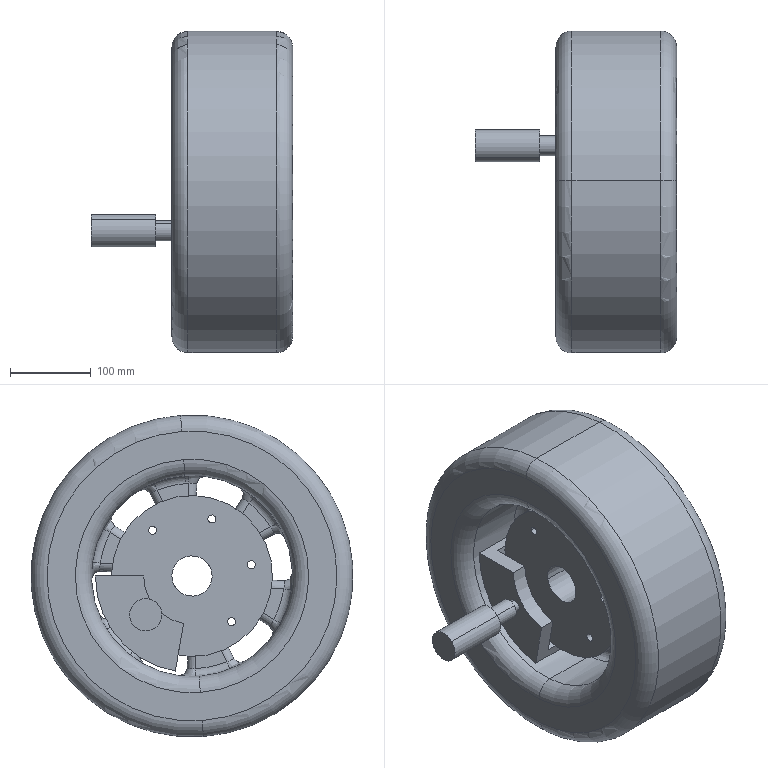Part | SolidWorks | features AEMSimFeature 1 | 7 solids | 245 faces | box 250 x 400 x 400 mm | volume 13503610 mm3 | cylinder 114 | torus 77 | plane 42 | spline 12 | commonest cylinder face diameters 20 x54 10 x12 30 x12 80 x6 15 x4 50 x4